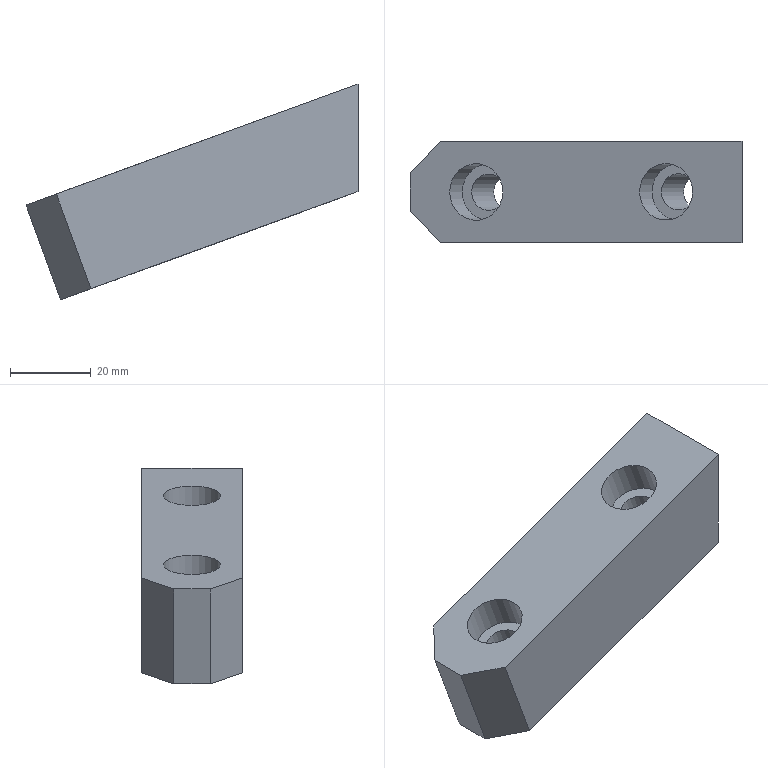Part | STEP file | P011002S003-009 | 1 solid | 14 faces | box 82.185 x 25 x 53.405 mm | volume 45412 mm3 | plane 10 | cylinder 4 | commonest cylinder face diameters 9 x2 14 x2
STEP:
#1=CARTESIAN_POINT('',(0.,0.,0.));
#2=DIRECTION('',(0.,0.,1.));
#3=DIRECTION('',(1.,0.,0.));
#4=AXIS2_PLACEMENT_3D('',#1,#2,#3);
#5=CARTESIAN_POINT('',(-226.457,-9.,-53.01));
#6=VERTEX_POINT('',#5);
#7=CARTESIAN_POINT('',(-217.999,-9.,-49.932));
#8=VERTEX_POINT('',#7);
#9=CARTESIAN_POINT('',(-222.228,-9.,-51.471));
#10=DIRECTION('',(0.342,0.,-0.9397));
#11=DIRECTION('',(-0.9397,0.,-0.342));
#12=AXIS2_PLACEMENT_3D('',#9,#10,#11);
#13=CIRCLE('',#12,4.5);
#14=CARTESIAN_POINT('',(-161.58,106.,-29.397));
#15=DIRECTION('',(0.342,0.,-0.9397));
#16=DIRECTION('',(0.9397,0.,0.342));
#17=AXIS2_PLACEMENT_3D('',#14,#15,#16);
#18=PLANE('',#17);
#19=CARTESIAN_POINT('',(-64.54,115.));
#20=DIRECTION('',(-1.,0.));
#21=AXIS2_PLACEMENT_2D('',#19,#20);
#22=CIRCLE('',#21,4.5);
#23=(GEOMETRIC_REPRESENTATION_CONTEXT(2)PARAMETRIC_REPRESENTATION_CONTEXT()REPRESENTATION_CONTEXT('',''));
#24=DEFINITIONAL_REPRESENTATION('',(#22),#23);
#25=PCURVE('',#18,#24);
#26=CARTESIAN_POINT('',(-230.778,-9.,-27.979));
#27=DIRECTION('',(0.342,0.,-0.9397));
#28=DIRECTION('',(0.9397,0.,0.342));
#29=AXIS2_PLACEMENT_3D('',#26,#27,#28);
#30=CYLINDRICAL_SURFACE('',#29,4.5);
#31=CARTESIAN_POINT('',(3.142,25.));
#32=DIRECTION('',(1.,0.));
#33=VECTOR('',#32,1.);
#34=LINE('',#31,#33);
#35=(GEOMETRIC_REPRESENTATION_CONTEXT(2)PARAMETRIC_REPRESENTATION_CONTEXT()REPRESENTATION_CONTEXT('',''));
#36=DEFINITIONAL_REPRESENTATION('',(#34),#35);
#37=PCURVE('',#30,#36);
#38=SURFACE_CURVE('',#13,(#25,#37),.PCURVE_S1.);
#39=EDGE_CURVE('',#6,#8,#38,.T.);
#40=ORIENTED_EDGE('',*,*,#39,.F.);
#41=CARTESIAN_POINT('',(-222.228,-9.,-51.471));
#42=DIRECTION('',(0.342,0.,-0.9397));
#43=DIRECTION('',(-0.9397,0.,-0.342));
#44=AXIS2_PLACEMENT_3D('',#41,#42,#43);
#45=CIRCLE('',#44,4.5);
#46=CARTESIAN_POINT('',(-64.54,115.));
#47=DIRECTION('',(-1.,0.));
#48=AXIS2_PLACEMENT_2D('',#46,#47);
#49=CIRCLE('',#48,4.5);
#50=(GEOMETRIC_REPRESENTATION_CONTEXT(2)PARAMETRIC_REPRESENTATION_CONTEXT()REPRESENTATION_CONTEXT('',''));
#51=DEFINITIONAL_REPRESENTATION('',(#49),#50);
#52=PCURVE('',#18,#51);
#53=CARTESIAN_POINT('',(-3.142,25.));
#54=DIRECTION('',(1.,0.));
#55=VECTOR('',#54,1.);
#56=LINE('',#53,#55);
#57=(GEOMETRIC_REPRESENTATION_CONTEXT(2)PARAMETRIC_REPRESENTATION_CONTEXT()REPRESENTATION_CONTEXT('',''));
#58=DEFINITIONAL_REPRESENTATION('',(#56),#57);
#59=PCURVE('',#30,#58);
#60=SURFACE_CURVE('',#45,(#52,#59),.PCURVE_S1.);
#61=EDGE_CURVE('',#8,#6,#60,.T.);
#62=ORIENTED_EDGE('',*,*,#61,.F.);
#63=EDGE_LOOP('',(#40,#62));
#64=FACE_BOUND('',#63,.T.);
#65=CARTESIAN_POINT('',(-165.,3.5,-30.642));
#66=VERTEX_POINT('',#65);
#67=CARTESIAN_POINT('',(-231.117,3.5,-54.706));
#68=VERTEX_POINT('',#67);
#69=CARTESIAN_POINT('',(-224.539,3.5,-52.312));
#70=DIRECTION('',(-0.9397,0.,-0.342));
#71=VECTOR('',#70,1.);
#72=LINE('',#69,#71);
#73=CARTESIAN_POINT('',(-67.,102.5));
#74=DIRECTION('',(-1.,0.));
#75=VECTOR('',#74,1.);
#76=LINE('',#73,#75);
#77=(GEOMETRIC_REPRESENTATION_CONTEXT(2)PARAMETRIC_REPRESENTATION_CONTEXT()REPRESENTATION_CONTEXT('',''));
#78=DEFINITIONAL_REPRESENTATION('',(#76),#77);
#79=PCURVE('',#18,#78);
#80=CARTESIAN_POINT('',(-229.67,3.5,-38.217));
#81=DIRECTION('',(0.,1.,0.));
#82=DIRECTION('',(0.9397,0.,0.342));
#83=AXIS2_PLACEMENT_3D('',#80,#81,#82);
#84=PLANE('',#83);
#85=CARTESIAN_POINT('',(0.,15.));
#86=DIRECTION('',(-1.,0.));
#87=VECTOR('',#86,1.);
#88=LINE('',#85,#87);
#89=(GEOMETRIC_REPRESENTATION_CONTEXT(2)PARAMETRIC_REPRESENTATION_CONTEXT()REPRESENTATION_CONTEXT('',''));
#90=DEFINITIONAL_REPRESENTATION('',(#88),#89);
#91=PCURVE('',#84,#90);
#92=SURFACE_CURVE('',#72,(#79,#91),.PCURVE_S1.);
#93=EDGE_CURVE('',#66,#68,#92,.T.);
#94=ORIENTED_EDGE('',*,*,#93,.F.);
#95=CARTESIAN_POINT('',(-165.,-21.5,-30.642));
#96=VERTEX_POINT('',#95);
#97=CARTESIAN_POINT('',(-165.,200.,-30.642));
#98=DIRECTION('',(0.,1.,0.));
#99=VECTOR('',#98,1.);
#100=LINE('',#97,#99);
#101=CARTESIAN_POINT('',(-3.64,-94.));
#102=DIRECTION('',(0.,-1.));
#103=VECTOR('',#102,1.);
#104=LINE('',#101,#103);
#105=(GEOMETRIC_REPRESENTATION_CONTEXT(2)PARAMETRIC_REPRESENTATION_CONTEXT()REPRESENTATION_CONTEXT('',''));
#106=DEFINITIONAL_REPRESENTATION('',(#104),#105);
#107=PCURVE('',#18,#106);
#108=CARTESIAN_POINT('',(-165.,200.,-50.));
#109=DIRECTION('',(1.,0.,0.));
#110=DIRECTION('',(0.,-1.,0.));
#111=AXIS2_PLACEMENT_3D('',#108,#109,#110);
#112=PLANE('',#111);
#113=CARTESIAN_POINT('',(0.,-19.358));
#114=DIRECTION('',(-1.,0.));
#115=VECTOR('',#114,1.);
#116=LINE('',#113,#115);
#117=(GEOMETRIC_REPRESENTATION_CONTEXT(2)PARAMETRIC_REPRESENTATION_CONTEXT()REPRESENTATION_CONTEXT('',''));
#118=DEFINITIONAL_REPRESENTATION('',(#116),#117);
#119=PCURVE('',#112,#118);
#120=SURFACE_CURVE('',#100,(#107,#119),.PCURVE_S1.);
#121=EDGE_CURVE('',#96,#66,#120,.T.);
#122=ORIENTED_EDGE('',*,*,#121,.F.);
#123=CARTESIAN_POINT('',(-231.117,-21.5,-54.706));
#124=VERTEX_POINT('',#123);
#125=CARTESIAN_POINT('',(-161.58,-21.5,-29.397));
#126=DIRECTION('',(-0.9397,0.,-0.342));
#127=VECTOR('',#126,1.);
#128=LINE('',#125,#127);
#129=CARTESIAN_POINT('',(0.,127.5));
#130=DIRECTION('',(-1.,0.));
#131=VECTOR('',#130,1.);
#132=LINE('',#129,#131);
#133=(GEOMETRIC_REPRESENTATION_CONTEXT(2)PARAMETRIC_REPRESENTATION_CONTEXT()REPRESENTATION_CONTEXT('',''));
#134=DEFINITIONAL_REPRESENTATION('',(#132),#133);
#135=PCURVE('',#18,#134);
#136=CARTESIAN_POINT('',(-229.67,-21.5,-38.217));
#137=DIRECTION('',(0.,-1.,0.));
#138=DIRECTION('',(-0.9397,0.,-0.342));
#139=AXIS2_PLACEMENT_3D('',#136,#137,#138);
#140=PLANE('',#139);
#141=CARTESIAN_POINT('',(-67.,15.));
#142=DIRECTION('',(1.,0.));
#143=VECTOR('',#142,1.);
#144=LINE('',#141,#143);
#145=(GEOMETRIC_REPRESENTATION_CONTEXT(2)PARAMETRIC_REPRESENTATION_CONTEXT()REPRESENTATION_CONTEXT('',''));
#146=DEFINITIONAL_REPRESENTATION('',(#144),#145);
#147=PCURVE('',#140,#146);
#148=SURFACE_CURVE('',#128,(#135,#147),.PCURVE_S1.);
#149=EDGE_CURVE('',#96,#124,#148,.T.);
#150=ORIENTED_EDGE('',*,*,#149,.T.);
#151=CARTESIAN_POINT('',(-238.635,-13.5,-57.443));
#152=VERTEX_POINT('',#151);
#153=CARTESIAN_POINT('',(-231.117,-21.5,-54.706));
#154=DIRECTION('',(0.6645,-0.7071,0.2418));
#155=VECTOR('',#154,1.);
#156=LINE('',#153,#155);
#157=CARTESIAN_POINT('',(-74.,127.5));
#158=DIRECTION('',(0.7071,0.7071));
#159=VECTOR('',#158,1.);
#160=LINE('',#157,#159);
#161=(GEOMETRIC_REPRESENTATION_CONTEXT(2)PARAMETRIC_REPRESENTATION_CONTEXT()REPRESENTATION_CONTEXT('',''));
#162=DEFINITIONAL_REPRESENTATION('',(#160),#161);
#163=PCURVE('',#18,#162);
#164=CARTESIAN_POINT('',(-236.247,-21.5,-40.611));
#165=DIRECTION('',(0.6645,0.7071,0.2418));
#166=DIRECTION('',(0.7287,-0.6848,0.));
#167=AXIS2_PLACEMENT_3D('',#164,#165,#166);
#168=PLANE('',#167);
#169=CARTESIAN_POINT('',(3.739,14.527));
#170=DIRECTION('',(0.9684,-0.2492));
#171=VECTOR('',#170,1.);
#172=LINE('',#169,#171);
#173=(GEOMETRIC_REPRESENTATION_CONTEXT(2)PARAMETRIC_REPRESENTATION_CONTEXT()REPRESENTATION_CONTEXT('',''));
#174=DEFINITIONAL_REPRESENTATION('',(#172),#173);
#175=PCURVE('',#168,#174);
#176=SURFACE_CURVE('',#156,(#163,#175),.PCURVE_S1.);
#177=EDGE_CURVE('',#152,#124,#176,.T.);
#178=ORIENTED_EDGE('',*,*,#177,.F.);
#179=CARTESIAN_POINT('',(-238.635,-4.5,-57.443));
#180=VERTEX_POINT('',#179);
#181=CARTESIAN_POINT('',(-238.635,-14.,-57.443));
#182=DIRECTION('',(0.,-1.,0.));
#183=VECTOR('',#182,1.);
#184=LINE('',#181,#183);
#185=CARTESIAN_POINT('',(-82.,120.));
#186=DIRECTION('',(0.,1.));
#187=VECTOR('',#186,1.);
#188=LINE('',#185,#187);
#189=(GEOMETRIC_REPRESENTATION_CONTEXT(2)PARAMETRIC_REPRESENTATION_CONTEXT()REPRESENTATION_CONTEXT('',''));
#190=DEFINITIONAL_REPRESENTATION('',(#188),#189);
#191=PCURVE('',#18,#190);
#192=CARTESIAN_POINT('',(-243.765,-14.,-43.347));
#193=DIRECTION('',(-0.9397,0.,-0.342));
#194=DIRECTION('',(-0.342,0.,0.9397));
#195=AXIS2_PLACEMENT_3D('',#192,#193,#194);
#196=PLANE('',#195);
#197=CARTESIAN_POINT('',(-15.,0.));
#198=DIRECTION('',(0.,-1.));
#199=VECTOR('',#198,1.);
#200=LINE('',#197,#199);
#201=(GEOMETRIC_REPRESENTATION_CONTEXT(2)PARAMETRIC_REPRESENTATION_CONTEXT()REPRESENTATION_CONTEXT('',''));
#202=DEFINITIONAL_REPRESENTATION('',(#200),#201);
#203=PCURVE('',#196,#202);
#204=SURFACE_CURVE('',#184,(#191,#203),.PCURVE_S1.);
#205=EDGE_CURVE('',#180,#152,#204,.T.);
#206=ORIENTED_EDGE('',*,*,#205,.F.);
#207=CARTESIAN_POINT('',(-231.117,3.5,-54.706));
#208=DIRECTION('',(-0.6645,-0.7071,-0.2418));
#209=VECTOR('',#208,1.);
#210=LINE('',#207,#209);
#211=CARTESIAN_POINT('',(-74.,102.5));
#212=DIRECTION('',(-0.7071,0.7071));
#213=VECTOR('',#212,1.);
#214=LINE('',#211,#213);
#215=(GEOMETRIC_REPRESENTATION_CONTEXT(2)PARAMETRIC_REPRESENTATION_CONTEXT()REPRESENTATION_CONTEXT('',''));
#216=DEFINITIONAL_REPRESENTATION('',(#214),#215);
#217=PCURVE('',#18,#216);
#218=CARTESIAN_POINT('',(-236.247,3.5,-40.611));
#219=DIRECTION('',(0.6645,-0.7071,0.2418));
#220=DIRECTION('',(-0.7287,-0.6848,0.));
#221=AXIS2_PLACEMENT_3D('',#218,#219,#220);
#222=PLANE('',#221);
#223=CARTESIAN_POINT('',(-3.739,14.527));
#224=DIRECTION('',(0.9684,0.2492));
#225=VECTOR('',#224,1.);
#226=LINE('',#223,#225);
#227=(GEOMETRIC_REPRESENTATION_CONTEXT(2)PARAMETRIC_REPRESENTATION_CONTEXT()REPRESENTATION_CONTEXT('',''));
#228=DEFINITIONAL_REPRESENTATION('',(#226),#227);
#229=PCURVE('',#222,#228);
#230=SURFACE_CURVE('',#210,(#217,#229),.PCURVE_S1.);
#231=EDGE_CURVE('',#68,#180,#230,.T.);
#232=ORIENTED_EDGE('',*,*,#231,.F.);
#233=EDGE_LOOP('',(#94,#122,#150,#178,#206,#232));
#234=FACE_BOUND('',#233,.T.);
#235=CARTESIAN_POINT('',(-179.472,-9.,-35.909));
#236=VERTEX_POINT('',#235);
#237=CARTESIAN_POINT('',(-171.015,-9.,-32.831));
#238=VERTEX_POINT('',#237);
#239=CARTESIAN_POINT('',(-175.243,-9.,-34.37));
#240=DIRECTION('',(0.342,0.,-0.9397));
#241=DIRECTION('',(-0.9397,0.,-0.342));
#242=AXIS2_PLACEMENT_3D('',#239,#240,#241);
#243=CIRCLE('',#242,4.5);
#244=CARTESIAN_POINT('',(-14.54,115.));
#245=DIRECTION('',(-1.,0.));
#246=AXIS2_PLACEMENT_2D('',#244,#245);
#247=CIRCLE('',#246,4.5);
#248=(GEOMETRIC_REPRESENTATION_CONTEXT(2)PARAMETRIC_REPRESENTATION_CONTEXT()REPRESENTATION_CONTEXT('',''));
#249=DEFINITIONAL_REPRESENTATION('',(#247),#248);
#250=PCURVE('',#18,#249);
#251=CARTESIAN_POINT('',(-183.794,-9.,-10.878));
#252=DIRECTION('',(0.342,0.,-0.9397));
#253=DIRECTION('',(0.9397,0.,0.342));
#254=AXIS2_PLACEMENT_3D('',#251,#252,#253);
#255=CYLINDRICAL_SURFACE('',#254,4.5);
#256=CARTESIAN_POINT('',(3.142,25.));
#257=DIRECTION('',(1.,0.));
#258=VECTOR('',#257,1.);
#259=LINE('',#256,#258);
#260=(GEOMETRIC_REPRESENTATION_CONTEXT(2)PARAMETRIC_REPRESENTATION_CONTEXT()REPRESENTATION_CONTEXT('',''));
#261=DEFINITIONAL_REPRESENTATION('',(#259),#260);
#262=PCURVE('',#255,#261);
#263=SURFACE_CURVE('',#243,(#250,#262),.PCURVE_S1.);
#264=EDGE_CURVE('',#236,#238,#263,.T.);
#265=ORIENTED_EDGE('',*,*,#264,.F.);
#266=CARTESIAN_POINT('',(-175.243,-9.,-34.37));
#267=DIRECTION('',(0.342,0.,-0.9397));
#268=DIRECTION('',(-0.9397,0.,-0.342));
#269=AXIS2_PLACEMENT_3D('',#266,#267,#268);
#270=CIRCLE('',#269,4.5);
#271=CARTESIAN_POINT('',(-14.54,115.));
#272=DIRECTION('',(-1.,0.));
#273=AXIS2_PLACEMENT_2D('',#271,#272);
#274=CIRCLE('',#273,4.5);
#275=(GEOMETRIC_REPRESENTATION_CONTEXT(2)PARAMETRIC_REPRESENTATION_CONTEXT()REPRESENTATION_CONTEXT('',''));
#276=DEFINITIONAL_REPRESENTATION('',(#274),#275);
#277=PCURVE('',#18,#276);
#278=CARTESIAN_POINT('',(-3.142,25.));
#279=DIRECTION('',(1.,0.));
#280=VECTOR('',#279,1.);
#281=LINE('',#278,#280);
#282=(GEOMETRIC_REPRESENTATION_CONTEXT(2)PARAMETRIC_REPRESENTATION_CONTEXT()REPRESENTATION_CONTEXT('',''));
#283=DEFINITIONAL_REPRESENTATION('',(#281),#282);
#284=PCURVE('',#255,#283);
#285=SURFACE_CURVE('',#270,(#277,#284),.PCURVE_S1.);
#286=EDGE_CURVE('',#238,#236,#285,.T.);
#287=ORIENTED_EDGE('',*,*,#286,.F.);
#288=EDGE_LOOP('',(#265,#287));
#289=FACE_BOUND('',#288,.T.);
#290=ADVANCED_FACE('',(#64,#234,#289),#18,.T.);
#291=ORIENTED_EDGE('',*,*,#205,.T.);
#292=CARTESIAN_POINT('',(-247.185,-13.5,-33.95));
#293=VERTEX_POINT('',#292);
#294=CARTESIAN_POINT('',(-243.765,-13.5,-43.347));
#295=DIRECTION('',(0.342,0.,-0.9397));
#296=VECTOR('',#295,1.);
#297=LINE('',#294,#296);
#298=CARTESIAN_POINT('',(0.,0.5));
#299=DIRECTION('',(-1.,0.));
#300=VECTOR('',#299,1.);
#301=LINE('',#298,#300);
#302=(GEOMETRIC_REPRESENTATION_CONTEXT(2)PARAMETRIC_REPRESENTATION_CONTEXT()REPRESENTATION_CONTEXT('',''));
#303=DEFINITIONAL_REPRESENTATION('',(#301),#302);
#304=PCURVE('',#196,#303);
#305=CARTESIAN_POINT('',(-10.957,2.82));
#306=DIRECTION('',(0.2492,0.9684));
#307=VECTOR('',#306,1.);
#308=LINE('',#305,#307);
#309=(GEOMETRIC_REPRESENTATION_CONTEXT(2)PARAMETRIC_REPRESENTATION_CONTEXT()REPRESENTATION_CONTEXT('',''));
#310=DEFINITIONAL_REPRESENTATION('',(#308),#309);
#311=PCURVE('',#168,#310);
#312=SURFACE_CURVE('',#297,(#304,#311),.PCURVE_S1.);
#313=EDGE_CURVE('',#293,#152,#312,.T.);
#314=ORIENTED_EDGE('',*,*,#313,.F.);
#315=CARTESIAN_POINT('',(-247.185,-4.5,-33.95));
#316=VERTEX_POINT('',#315);
#317=CARTESIAN_POINT('',(-247.185,-14.,-33.95));
#318=DIRECTION('',(0.,1.,0.));
#319=VECTOR('',#318,1.);
#320=LINE('',#317,#319);
#321=CARTESIAN_POINT('',(10.,0.));
#322=DIRECTION('',(0.,1.));
#323=VECTOR('',#322,1.);
#324=LINE('',#321,#323);
#325=(GEOMETRIC_REPRESENTATION_CONTEXT(2)PARAMETRIC_REPRESENTATION_CONTEXT()REPRESENTATION_CONTEXT('',''));
#326=DEFINITIONAL_REPRESENTATION('',(#324),#325);
#327=PCURVE('',#196,#326);
#328=CARTESIAN_POINT('',(-233.09,-14.,-28.82));
#329=DIRECTION('',(-0.342,0.,0.9397));
#330=DIRECTION('',(0.9397,0.,0.342));
#331=AXIS2_PLACEMENT_3D('',#328,#329,#330);
#332=PLANE('',#331);
#333=CARTESIAN_POINT('',(-15.,0.));
#334=DIRECTION('',(0.,1.));
#335=VECTOR('',#334,1.);
#336=LINE('',#333,#335);
#337=(GEOMETRIC_REPRESENTATION_CONTEXT(2)PARAMETRIC_REPRESENTATION_CONTEXT()REPRESENTATION_CONTEXT('',''));
#338=DEFINITIONAL_REPRESENTATION('',(#336),#337);
#339=PCURVE('',#332,#338);
#340=SURFACE_CURVE('',#320,(#327,#339),.PCURVE_S1.);
#341=EDGE_CURVE('',#293,#316,#340,.T.);
#342=ORIENTED_EDGE('',*,*,#341,.T.);
#343=CARTESIAN_POINT('',(-243.765,-4.5,-43.347));
#344=DIRECTION('',(-0.342,0.,0.9397));
#345=VECTOR('',#344,1.);
#346=LINE('',#343,#345);
#347=CARTESIAN_POINT('',(0.,9.5));
#348=DIRECTION('',(1.,0.));
#349=VECTOR('',#348,1.);
#350=LINE('',#347,#349);
#351=(GEOMETRIC_REPRESENTATION_CONTEXT(2)PARAMETRIC_REPRESENTATION_CONTEXT()REPRESENTATION_CONTEXT('',''));
#352=DEFINITIONAL_REPRESENTATION('',(#350),#351);
#353=PCURVE('',#196,#352);
#354=CARTESIAN_POINT('',(10.957,2.82));
#355=DIRECTION('',(0.2492,-0.9684));
#356=VECTOR('',#355,1.);
#357=LINE('',#354,#356);
#358=(GEOMETRIC_REPRESENTATION_CONTEXT(2)PARAMETRIC_REPRESENTATION_CONTEXT()REPRESENTATION_CONTEXT('',''));
#359=DEFINITIONAL_REPRESENTATION('',(#357),#358);
#360=PCURVE('',#222,#359);
#361=SURFACE_CURVE('',#346,(#353,#360),.PCURVE_S1.);
#362=EDGE_CURVE('',#180,#316,#361,.T.);
#363=ORIENTED_EDGE('',*,*,#362,.F.);
#364=EDGE_LOOP('',(#291,#314,#342,#363));
#365=FACE_BOUND('',#364,.T.);
#366=ADVANCED_FACE('',(#365),#196,.T.);
#367=CARTESIAN_POINT('',(-165.,3.5,-4.037));
#368=VERTEX_POINT('',#367);
#369=CARTESIAN_POINT('',(-239.668,3.5,-31.214));
#370=VERTEX_POINT('',#369);
#371=CARTESIAN_POINT('',(-233.09,3.5,-28.82));
#372=DIRECTION('',(-0.9397,0.,-0.342));
#373=VECTOR('',#372,1.);
#374=LINE('',#371,#373);
#375=CARTESIAN_POINT('',(0.,-10.));
#376=DIRECTION('',(-1.,0.));
#377=VECTOR('',#376,1.);
#378=LINE('',#375,#377);
#379=(GEOMETRIC_REPRESENTATION_CONTEXT(2)PARAMETRIC_REPRESENTATION_CONTEXT()REPRESENTATION_CONTEXT('',''));
#380=DEFINITIONAL_REPRESENTATION('',(#378),#379);
#381=PCURVE('',#84,#380);
#382=CARTESIAN_POINT('',(0.,17.5));
#383=DIRECTION('',(-1.,0.));
#384=VECTOR('',#383,1.);
#385=LINE('',#382,#384);
#386=(GEOMETRIC_REPRESENTATION_CONTEXT(2)PARAMETRIC_REPRESENTATION_CONTEXT()REPRESENTATION_CONTEXT('',''));
#387=DEFINITIONAL_REPRESENTATION('',(#385),#386);
#388=PCURVE('',#332,#387);
#389=SURFACE_CURVE('',#374,(#381,#388),.PCURVE_S1.);
#390=EDGE_CURVE('',#368,#370,#389,.T.);
#391=ORIENTED_EDGE('',*,*,#390,.F.);
#392=CARTESIAN_POINT('',(-165.,3.5,-38.217));
#393=DIRECTION('',(0.,0.,1.));
#394=VECTOR('',#393,1.);
#395=LINE('',#392,#394);
#396=CARTESIAN_POINT('',(60.769,22.118));
#397=DIRECTION('',(0.342,-0.9397));
#398=VECTOR('',#397,1.);
#399=LINE('',#396,#398);
#400=(GEOMETRIC_REPRESENTATION_CONTEXT(2)PARAMETRIC_REPRESENTATION_CONTEXT()REPRESENTATION_CONTEXT('',''));
#401=DEFINITIONAL_REPRESENTATION('',(#399),#400);
#402=PCURVE('',#84,#401);
#403=CARTESIAN_POINT('',(196.5,-11.783));
#404=DIRECTION('',(0.,-1.));
#405=VECTOR('',#404,1.);
#406=LINE('',#403,#405);
#407=(GEOMETRIC_REPRESENTATION_CONTEXT(2)PARAMETRIC_REPRESENTATION_CONTEXT()REPRESENTATION_CONTEXT('',''));
#408=DEFINITIONAL_REPRESENTATION('',(#406),#407);
#409=PCURVE('',#112,#408);
#410=SURFACE_CURVE('',#395,(#402,#409),.PCURVE_S1.);
#411=EDGE_CURVE('',#66,#368,#410,.T.);
#412=ORIENTED_EDGE('',*,*,#411,.F.);
#413=ORIENTED_EDGE('',*,*,#93,.T.);
#414=CARTESIAN_POINT('',(-236.247,3.5,-40.611));
#415=DIRECTION('',(0.342,0.,-0.9397));
#416=VECTOR('',#415,1.);
#417=LINE('',#414,#416);
#418=CARTESIAN_POINT('',(-7.,0.));
#419=DIRECTION('',(0.,1.));
#420=VECTOR('',#419,1.);
#421=LINE('',#418,#420);
#422=(GEOMETRIC_REPRESENTATION_CONTEXT(2)PARAMETRIC_REPRESENTATION_CONTEXT()REPRESENTATION_CONTEXT('',''));
#423=DEFINITIONAL_REPRESENTATION('',(#421),#422);
#424=PCURVE('',#84,#423);
#425=CARTESIAN_POINT('',(0.,0.));
#426=DIRECTION('',(-0.2492,0.9684));
#427=VECTOR('',#426,1.);
#428=LINE('',#425,#427);
#429=(GEOMETRIC_REPRESENTATION_CONTEXT(2)PARAMETRIC_REPRESENTATION_CONTEXT()REPRESENTATION_CONTEXT('',''));
#430=DEFINITIONAL_REPRESENTATION('',(#428),#429);
#431=PCURVE('',#222,#430);
#432=SURFACE_CURVE('',#417,(#424,#431),.PCURVE_S1.);
#433=EDGE_CURVE('',#370,#68,#432,.T.);
#434=ORIENTED_EDGE('',*,*,#433,.F.);
#435=EDGE_LOOP('',(#391,#412,#413,#434));
#436=FACE_BOUND('',#435,.T.);
#437=ADVANCED_FACE('',(#436),#84,.T.);
#438=ORIENTED_EDGE('',*,*,#149,.F.);
#439=CARTESIAN_POINT('',(-165.,-21.5,-4.037));
#440=VERTEX_POINT('',#439);
#441=CARTESIAN_POINT('',(-165.,-21.5,-38.217));
#442=DIRECTION('',(0.,0.,-1.));
#443=VECTOR('',#442,1.);
#444=LINE('',#441,#443);
#445=CARTESIAN_POINT('',(-60.769,22.118));
#446=DIRECTION('',(0.342,0.9397));
#447=VECTOR('',#446,1.);
#448=LINE('',#445,#447);
#449=(GEOMETRIC_REPRESENTATION_CONTEXT(2)PARAMETRIC_REPRESENTATION_CONTEXT()REPRESENTATION_CONTEXT('',''));
#450=DEFINITIONAL_REPRESENTATION('',(#448),#449);
#451=PCURVE('',#140,#450);
#452=CARTESIAN_POINT('',(221.5,-11.783));
#453=DIRECTION('',(0.,1.));
#454=VECTOR('',#453,1.);
#455=LINE('',#452,#454);
#456=(GEOMETRIC_REPRESENTATION_CONTEXT(2)PARAMETRIC_REPRESENTATION_CONTEXT()REPRESENTATION_CONTEXT('',''));
#457=DEFINITIONAL_REPRESENTATION('',(#455),#456);
#458=PCURVE('',#112,#457);
#459=SURFACE_CURVE('',#444,(#451,#458),.PCURVE_S1.);
#460=EDGE_CURVE('',#440,#96,#459,.T.);
#461=ORIENTED_EDGE('',*,*,#460,.F.);
#462=CARTESIAN_POINT('',(-239.668,-21.5,-31.214));
#463=VERTEX_POINT('',#462);
#464=CARTESIAN_POINT('',(-233.09,-21.5,-28.82));
#465=DIRECTION('',(-0.9397,0.,-0.342));
#466=VECTOR('',#465,1.);
#467=LINE('',#464,#466);
#468=CARTESIAN_POINT('',(0.,-10.));
#469=DIRECTION('',(1.,0.));
#470=VECTOR('',#469,1.);
#471=LINE('',#468,#470);
#472=(GEOMETRIC_REPRESENTATION_CONTEXT(2)PARAMETRIC_REPRESENTATION_CONTEXT()REPRESENTATION_CONTEXT('',''));
#473=DEFINITIONAL_REPRESENTATION('',(#471),#472);
#474=PCURVE('',#140,#473);
#475=CARTESIAN_POINT('',(0.,-7.5));
#476=DIRECTION('',(-1.,0.));
#477=VECTOR('',#476,1.);
#478=LINE('',#475,#477);
#479=(GEOMETRIC_REPRESENTATION_CONTEXT(2)PARAMETRIC_REPRESENTATION_CONTEXT()REPRESENTATION_CONTEXT('',''));
#480=DEFINITIONAL_REPRESENTATION('',(#478),#479);
#481=PCURVE('',#332,#480);
#482=SURFACE_CURVE('',#467,(#474,#481),.PCURVE_S1.);
#483=EDGE_CURVE('',#440,#463,#482,.T.);
#484=ORIENTED_EDGE('',*,*,#483,.T.);
#485=CARTESIAN_POINT('',(-236.247,-21.5,-40.611));
#486=DIRECTION('',(-0.342,0.,0.9397));
#487=VECTOR('',#486,1.);
#488=LINE('',#485,#487);
#489=CARTESIAN_POINT('',(7.,0.));
#490=DIRECTION('',(0.,-1.));
#491=VECTOR('',#490,1.);
#492=LINE('',#489,#491);
#493=(GEOMETRIC_REPRESENTATION_CONTEXT(2)PARAMETRIC_REPRESENTATION_CONTEXT()REPRESENTATION_CONTEXT('',''));
#494=DEFINITIONAL_REPRESENTATION('',(#492),#493);
#495=PCURVE('',#140,#494);
#496=CARTESIAN_POINT('',(0.,0.));
#497=DIRECTION('',(-0.2492,-0.9684));
#498=VECTOR('',#497,1.);
#499=LINE('',#496,#498);
#500=(GEOMETRIC_REPRESENTATION_CONTEXT(2)PARAMETRIC_REPRESENTATION_CONTEXT()REPRESENTATION_CONTEXT('',''));
#501=DEFINITIONAL_REPRESENTATION('',(#499),#500);
#502=PCURVE('',#168,#501);
#503=SURFACE_CURVE('',#488,(#495,#502),.PCURVE_S1.);
#504=EDGE_CURVE('',#124,#463,#503,.T.);
#505=ORIENTED_EDGE('',*,*,#504,.F.);
#506=EDGE_LOOP('',(#438,#461,#484,#505));
#507=FACE_BOUND('',#506,.T.);
#508=ADVANCED_FACE('',(#507),#140,.T.);
#509=CARTESIAN_POINT('',(-165.,-14.,-4.037));
#510=DIRECTION('',(0.,-1.,0.));
#511=VECTOR('',#510,1.);
#512=LINE('',#509,#511);
#513=CARTESIAN_POINT('',(214.,-45.963));
#514=DIRECTION('',(1.,0.));
#515=VECTOR('',#514,1.);
#516=LINE('',#513,#515);
#517=(GEOMETRIC_REPRESENTATION_CONTEXT(2)PARAMETRIC_REPRESENTATION_CONTEXT()REPRESENTATION_CONTEXT('',''));
#518=DEFINITIONAL_REPRESENTATION('',(#516),#517);
#519=PCURVE('',#112,#518);
#520=CARTESIAN_POINT('',(72.46,0.));
#521=DIRECTION('',(0.,-1.));
#522=VECTOR('',#521,1.);
#523=LINE('',#520,#522);
#524=(GEOMETRIC_REPRESENTATION_CONTEXT(2)PARAMETRIC_REPRESENTATION_CONTEXT()REPRESENTATION_CONTEXT('',''));
#525=DEFINITIONAL_REPRESENTATION('',(#523),#524);
#526=PCURVE('',#332,#525);
#527=SURFACE_CURVE('',#512,(#519,#526),.PCURVE_S1.);
#528=EDGE_CURVE('',#368,#440,#527,.T.);
#529=ORIENTED_EDGE('',*,*,#528,.T.);
#530=ORIENTED_EDGE('',*,*,#460,.T.);
#531=ORIENTED_EDGE('',*,*,#121,.T.);
#532=ORIENTED_EDGE('',*,*,#411,.T.);
#533=EDGE_LOOP('',(#529,#530,#531,#532));
#534=FACE_BOUND('',#533,.T.);
#535=ADVANCED_FACE('',(#534),#112,.T.);
#536=CARTESIAN_POINT('',(-224.201,-9.,-25.585));
#537=VERTEX_POINT('',#536);
#538=CARTESIAN_POINT('',(-230.778,-9.,-27.979));
#539=DIRECTION('',(0.342,0.,-0.9397));
#540=DIRECTION('',(0.9397,0.,0.342));
#541=AXIS2_PLACEMENT_3D('',#538,#539,#540);
#542=CIRCLE('',#541,7.);
#543=CARTESIAN_POINT('',(9.46,5.));
#544=CARTESIAN_POINT('',(9.46,-7.124));
#545=CARTESIAN_POINT('',(-1.04,-1.062));
#546=CARTESIAN_POINT('',(-11.54,5.));
#547=CARTESIAN_POINT('',(-1.04,11.062));
#548=CARTESIAN_POINT('',(9.46,17.124));
#549=CARTESIAN_POINT('',(9.46,5.));
#550=(BOUNDED_CURVE()B_SPLINE_CURVE(2,(#543,#544,#545,#546,#547,#548,#549),.UNSPECIFIED.,.T.,.F.)B_SPLINE_CURVE_WITH_KNOTS((1,2,2,2,2,1),(-2.094,0.,2.094,4.189,6.283,8.378),.UNSPECIFIED.)CURVE()GEOMETRIC_REPRESENTATION_ITEM()RATIONAL_B_SPLINE_CURVE((1.,0.5,1.,0.5,1.,0.5,1.))REPRESENTATION_ITEM(''));
#551=(GEOMETRIC_REPRESENTATION_CONTEXT(2)PARAMETRIC_REPRESENTATION_CONTEXT()REPRESENTATION_CONTEXT('',''));
#552=DEFINITIONAL_REPRESENTATION('',(#550),#551);
#553=PCURVE('',#332,#552);
#554=CARTESIAN_POINT('',(-230.778,-9.,-27.979));
#555=DIRECTION('',(0.342,0.,-0.9397));
#556=DIRECTION('',(0.9397,0.,0.342));
#557=AXIS2_PLACEMENT_3D('',#554,#555,#556);
#558=CYLINDRICAL_SURFACE('',#557,7.);
#559=CARTESIAN_POINT('',(0.,0.));
#560=DIRECTION('',(1.,0.));
#561=VECTOR('',#560,1.);
#562=LINE('',#559,#561);
#563=(GEOMETRIC_REPRESENTATION_CONTEXT(2)PARAMETRIC_REPRESENTATION_CONTEXT()REPRESENTATION_CONTEXT('',''));
#564=DEFINITIONAL_REPRESENTATION('',(#562),#563);
#565=PCURVE('',#558,#564);
#566=SURFACE_CURVE('',#542,(#553,#565),.PCURVE_S1.);
#567=EDGE_CURVE('',#537,#537,#566,.T.);
#568=ORIENTED_EDGE('',*,*,#567,.T.);
#569=EDGE_LOOP('',(#568));
#570=FACE_BOUND('',#569,.T.);
#571=CARTESIAN_POINT('',(-177.216,-9.,-8.484));
#572=VERTEX_POINT('',#571);
#573=CARTESIAN_POINT('',(-183.794,-9.,-10.878));
#574=DIRECTION('',(0.342,0.,-0.9397));
#575=DIRECTION('',(0.9397,0.,0.342));
#576=AXIS2_PLACEMENT_3D('',#573,#574,#575);
#577=CIRCLE('',#576,7.);
#578=CARTESIAN_POINT('',(59.46,5.));
#579=CARTESIAN_POINT('',(59.46,-7.124));
#580=CARTESIAN_POINT('',(48.96,-1.062));
#581=CARTESIAN_POINT('',(38.46,5.));
#582=CARTESIAN_POINT('',(48.96,11.062));
#583=CARTESIAN_POINT('',(59.46,17.124));
#584=CARTESIAN_POINT('',(59.46,5.));
#585=(BOUNDED_CURVE()B_SPLINE_CURVE(2,(#578,#579,#580,#581,#582,#583,#584),.UNSPECIFIED.,.T.,.F.)B_SPLINE_CURVE_WITH_KNOTS((1,2,2,2,2,1),(-2.094,0.,2.094,4.189,6.283,8.378),.UNSPECIFIED.)CURVE()GEOMETRIC_REPRESENTATION_ITEM()RATIONAL_B_SPLINE_CURVE((1.,0.5,1.,0.5,1.,0.5,1.))REPRESENTATION_ITEM(''));
#586=(GEOMETRIC_REPRESENTATION_CONTEXT(2)PARAMETRIC_REPRESENTATION_CONTEXT()REPRESENTATION_CONTEXT('',''));
#587=DEFINITIONAL_REPRESENTATION('',(#585),#586);
#588=PCURVE('',#332,#587);
#589=CARTESIAN_POINT('',(-183.794,-9.,-10.878));
#590=DIRECTION('',(0.342,0.,-0.9397));
#591=DIRECTION('',(0.9397,0.,0.342));
#592=AXIS2_PLACEMENT_3D('',#589,#590,#591);
#593=CYLINDRICAL_SURFACE('',#592,7.);
#594=CARTESIAN_POINT('',(0.,0.));
#595=DIRECTION('',(1.,0.));
#596=VECTOR('',#595,1.);
#597=LINE('',#594,#596);
#598=(GEOMETRIC_REPRESENTATION_CONTEXT(2)PARAMETRIC_REPRESENTATION_CONTEXT()REPRESENTATION_CONTEXT('',''));
#599=DEFINITIONAL_REPRESENTATION('',(#597),#598);
#600=PCURVE('',#593,#599);
#601=SURFACE_CURVE('',#577,(#588,#600),.PCURVE_S1.);
#602=EDGE_CURVE('',#572,#572,#601,.T.);
#603=ORIENTED_EDGE('',*,*,#602,.T.);
#604=EDGE_LOOP('',(#603));
#605=FACE_BOUND('',#604,.T.);
#606=ORIENTED_EDGE('',*,*,#341,.F.);
#607=CARTESIAN_POINT('',(-239.902,-21.25,-31.3));
#608=DIRECTION('',(-0.6645,0.7071,-0.2418));
#609=VECTOR('',#608,1.);
#610=LINE('',#607,#609);
#611=CARTESIAN_POINT('',(-7.25,-7.25));
#612=DIRECTION('',(-0.7071,0.7071));
#613=VECTOR('',#612,1.);
#614=LINE('',#611,#613);
#615=(GEOMETRIC_REPRESENTATION_CONTEXT(2)PARAMETRIC_REPRESENTATION_CONTEXT()REPRESENTATION_CONTEXT('',''));
#616=DEFINITIONAL_REPRESENTATION('',(#614),#615);
#617=PCURVE('',#332,#616);
#618=CARTESIAN_POINT('',(-2.835,-9.596));
#619=DIRECTION('',(-0.9684,0.2492));
#620=VECTOR('',#619,1.);
#621=LINE('',#618,#620);
#622=(GEOMETRIC_REPRESENTATION_CONTEXT(2)PARAMETRIC_REPRESENTATION_CONTEXT()REPRESENTATION_CONTEXT('',''));
#623=DEFINITIONAL_REPRESENTATION('',(#621),#622);
#624=PCURVE('',#168,#623);
#625=SURFACE_CURVE('',#610,(#617,#624),.PCURVE_S1.);
#626=EDGE_CURVE('',#463,#293,#625,.T.);
#627=ORIENTED_EDGE('',*,*,#626,.F.);
#628=ORIENTED_EDGE('',*,*,#483,.F.);
#629=ORIENTED_EDGE('',*,*,#528,.F.);
#630=ORIENTED_EDGE('',*,*,#390,.T.);
#631=CARTESIAN_POINT('',(-244.601,-1.75,-33.01));
#632=DIRECTION('',(0.6645,0.7071,0.2418));
#633=VECTOR('',#632,1.);
#634=LINE('',#631,#633);
#635=CARTESIAN_POINT('',(-12.25,12.25));
#636=DIRECTION('',(0.7071,0.7071));
#637=VECTOR('',#636,1.);
#638=LINE('',#635,#637);
#639=(GEOMETRIC_REPRESENTATION_CONTEXT(2)PARAMETRIC_REPRESENTATION_CONTEXT()REPRESENTATION_CONTEXT('',''));
#640=DEFINITIONAL_REPRESENTATION('',(#638),#639);
#641=PCURVE('',#332,#640);
#642=CARTESIAN_POINT('',(9.683,-7.834));
#643=DIRECTION('',(-0.9684,-0.2492));
#644=VECTOR('',#643,1.);
#645=LINE('',#642,#644);
#646=(GEOMETRIC_REPRESENTATION_CONTEXT(2)PARAMETRIC_REPRESENTATION_CONTEXT()REPRESENTATION_CONTEXT('',''));
#647=DEFINITIONAL_REPRESENTATION('',(#645),#646);
#648=PCURVE('',#222,#647);
#649=SURFACE_CURVE('',#634,(#641,#648),.PCURVE_S1.);
#650=EDGE_CURVE('',#316,#370,#649,.T.);
#651=ORIENTED_EDGE('',*,*,#650,.F.);
#652=EDGE_LOOP('',(#606,#627,#628,#629,#630,#651));
#653=FACE_BOUND('',#652,.T.);
#654=ADVANCED_FACE('',(#570,#605,#653),#332,.T.);
#655=ORIENTED_EDGE('',*,*,#650,.T.);
#656=ORIENTED_EDGE('',*,*,#433,.T.);
#657=ORIENTED_EDGE('',*,*,#231,.T.);
#658=ORIENTED_EDGE('',*,*,#362,.T.);
#659=EDGE_LOOP('',(#655,#656,#657,#658));
#660=FACE_BOUND('',#659,.T.);
#661=ADVANCED_FACE('',(#660),#222,.F.);
#662=ORIENTED_EDGE('',*,*,#177,.T.);
#663=ORIENTED_EDGE('',*,*,#504,.T.);
#664=ORIENTED_EDGE('',*,*,#626,.T.);
#665=ORIENTED_EDGE('',*,*,#313,.T.);
#666=EDGE_LOOP('',(#662,#663,#664,#665));
#667=FACE_BOUND('',#666,.T.);
#668=ADVANCED_FACE('',(#667),#168,.F.);
#669=ORIENTED_EDGE('',*,*,#286,.F.);
#670=CARTESIAN_POINT('',(-176.487,-9.,-17.796));
#671=VERTEX_POINT('',#670);
#672=CARTESIAN_POINT('',(-176.487,-9.,-17.796));
#673=CARTESIAN_POINT('',(-171.015,-9.,-32.831));
#674=B_SPLINE_CURVE_WITH_KNOTS('',1,(#672,#673),.UNSPECIFIED.,.F.,.F.,(2,2),(9.,25.),.PIECEWISE_BEZIER_KNOTS.);
#675=CARTESIAN_POINT('',(0.,0.));
#676=DIRECTION('',(0.,1.));
#677=VECTOR('',#676,1.);
#678=LINE('',#675,#677);
#679=(GEOMETRIC_REPRESENTATION_CONTEXT(2)PARAMETRIC_REPRESENTATION_CONTEXT()REPRESENTATION_CONTEXT('',''));
#680=DEFINITIONAL_REPRESENTATION('',(#678),#679);
#681=PCURVE('',#255,#680);
#682=CARTESIAN_POINT('',(6.283,0.));
#683=DIRECTION('',(0.,1.));
#684=VECTOR('',#683,1.);
#685=LINE('',#682,#684);
#686=(GEOMETRIC_REPRESENTATION_CONTEXT(2)PARAMETRIC_REPRESENTATION_CONTEXT()REPRESENTATION_CONTEXT('',''));
#687=DEFINITIONAL_REPRESENTATION('',(#685),#686);
#688=PCURVE('',#255,#687);
#689=SEAM_CURVE('',#674,(#681,#688),.PCURVE_S1.);
#690=EDGE_CURVE('',#671,#238,#689,.T.);
#691=ORIENTED_EDGE('',*,*,#690,.F.);
#692=CARTESIAN_POINT('',(-180.716,-9.,-19.335));
#693=DIRECTION('',(-0.342,0.,0.9397));
#694=DIRECTION('',(0.9397,0.,0.342));
#695=AXIS2_PLACEMENT_3D('',#692,#693,#694);
#696=CIRCLE('',#695,4.5);
#697=CARTESIAN_POINT('',(6.283,9.));
#698=DIRECTION('',(-1.,0.));
#699=VECTOR('',#698,1.);
#700=LINE('',#697,#699);
#701=(GEOMETRIC_REPRESENTATION_CONTEXT(2)PARAMETRIC_REPRESENTATION_CONTEXT()REPRESENTATION_CONTEXT('',''));
#702=DEFINITIONAL_REPRESENTATION('',(#700),#701);
#703=PCURVE('',#255,#702);
#704=CARTESIAN_POINT('',(-176.017,-9.,-17.625));
#705=DIRECTION('',(0.342,0.,-0.9397));
#706=DIRECTION('',(0.9397,0.,0.342));
#707=AXIS2_PLACEMENT_3D('',#704,#705,#706);
#708=PLANE('',#707);
#709=CARTESIAN_POINT('',(-0.5,0.));
#710=CARTESIAN_POINT('',(-0.5,-7.794));
#711=CARTESIAN_POINT('',(-7.25,-3.897));
#712=CARTESIAN_POINT('',(-14.,0.));
#713=CARTESIAN_POINT('',(-7.25,3.897));
#714=CARTESIAN_POINT('',(-0.5,7.794));
#715=CARTESIAN_POINT('',(-0.5,0.));
#716=(BOUNDED_CURVE()B_SPLINE_CURVE(2,(#709,#710,#711,#712,#713,#714,#715),.UNSPECIFIED.,.T.,.F.)B_SPLINE_CURVE_WITH_KNOTS((1,2,2,2,2,1),(-2.094,0.,2.094,4.189,6.283,8.378),.UNSPECIFIED.)CURVE()GEOMETRIC_REPRESENTATION_ITEM()RATIONAL_B_SPLINE_CURVE((1.,0.5,1.,0.5,1.,0.5,1.))REPRESENTATION_ITEM(''));
#717=(GEOMETRIC_REPRESENTATION_CONTEXT(2)PARAMETRIC_REPRESENTATION_CONTEXT()REPRESENTATION_CONTEXT('',''));
#718=DEFINITIONAL_REPRESENTATION('',(#716),#717);
#719=PCURVE('',#708,#718);
#720=SURFACE_CURVE('',#696,(#703,#719),.PCURVE_S1.);
#721=EDGE_CURVE('',#671,#671,#720,.T.);
#722=ORIENTED_EDGE('',*,*,#721,.F.);
#723=ORIENTED_EDGE('',*,*,#690,.T.);
#724=ORIENTED_EDGE('',*,*,#264,.F.);
#725=EDGE_LOOP('',(#669,#691,#722,#723,#724));
#726=FACE_BOUND('',#725,.F.);
#727=ADVANCED_FACE('',(#726),#255,.F.);
#728=CARTESIAN_POINT('',(-174.138,-9.,-16.941));
#729=VERTEX_POINT('',#728);
#730=CARTESIAN_POINT('',(-180.716,-9.,-19.335));
#731=DIRECTION('',(-0.342,0.,0.9397));
#732=DIRECTION('',(0.9397,0.,0.342));
#733=AXIS2_PLACEMENT_3D('',#730,#731,#732);
#734=CIRCLE('',#733,7.);
#735=CARTESIAN_POINT('',(2.,0.));
#736=CARTESIAN_POINT('',(2.,-12.124));
#737=CARTESIAN_POINT('',(-8.5,-6.062));
#738=CARTESIAN_POINT('',(-19.,0.));
#739=CARTESIAN_POINT('',(-8.5,6.062));
#740=CARTESIAN_POINT('',(2.,12.124));
#741=CARTESIAN_POINT('',(2.,0.));
#742=(BOUNDED_CURVE()B_SPLINE_CURVE(2,(#735,#736,#737,#738,#739,#740,#741),.UNSPECIFIED.,.T.,.F.)B_SPLINE_CURVE_WITH_KNOTS((1,2,2,2,2,1),(-2.094,0.,2.094,4.189,6.283,8.378),.UNSPECIFIED.)CURVE()GEOMETRIC_REPRESENTATION_ITEM()RATIONAL_B_SPLINE_CURVE((1.,0.5,1.,0.5,1.,0.5,1.))REPRESENTATION_ITEM(''));
#743=(GEOMETRIC_REPRESENTATION_CONTEXT(2)PARAMETRIC_REPRESENTATION_CONTEXT()REPRESENTATION_CONTEXT('',''));
#744=DEFINITIONAL_REPRESENTATION('',(#742),#743);
#745=PCURVE('',#708,#744);
#746=CARTESIAN_POINT('',(6.283,9.));
#747=DIRECTION('',(-1.,0.));
#748=VECTOR('',#747,1.);
#749=LINE('',#746,#748);
#750=(GEOMETRIC_REPRESENTATION_CONTEXT(2)PARAMETRIC_REPRESENTATION_CONTEXT()REPRESENTATION_CONTEXT('',''));
#751=DEFINITIONAL_REPRESENTATION('',(#749),#750);
#752=PCURVE('',#593,#751);
#753=SURFACE_CURVE('',#734,(#745,#752),.PCURVE_S1.);
#754=EDGE_CURVE('',#729,#729,#753,.T.);
#755=ORIENTED_EDGE('',*,*,#754,.T.);
#756=EDGE_LOOP('',(#755));
#757=FACE_BOUND('',#756,.T.);
#758=ORIENTED_EDGE('',*,*,#721,.F.);
#759=EDGE_LOOP('',(#758));
#760=FACE_BOUND('',#759,.T.);
#761=ADVANCED_FACE('',(#757,#760),#708,.F.);
#762=ORIENTED_EDGE('',*,*,#602,.T.);
#763=CARTESIAN_POINT('',(-177.216,-9.,-8.484));
#764=CARTESIAN_POINT('',(-174.138,-9.,-16.941));
#765=B_SPLINE_CURVE_WITH_KNOTS('',1,(#763,#764),.UNSPECIFIED.,.F.,.F.,(2,2),(0.,9.),.PIECEWISE_BEZIER_KNOTS.);
#766=CARTESIAN_POINT('',(6.283,0.));
#767=DIRECTION('',(0.,1.));
#768=VECTOR('',#767,1.);
#769=LINE('',#766,#768);
#770=(GEOMETRIC_REPRESENTATION_CONTEXT(2)PARAMETRIC_REPRESENTATION_CONTEXT()REPRESENTATION_CONTEXT('',''));
#771=DEFINITIONAL_REPRESENTATION('',(#769),#770);
#772=PCURVE('',#593,#771);
#773=CARTESIAN_POINT('',(0.,0.));
#774=DIRECTION('',(0.,1.));
#775=VECTOR('',#774,1.);
#776=LINE('',#773,#775);
#777=(GEOMETRIC_REPRESENTATION_CONTEXT(2)PARAMETRIC_REPRESENTATION_CONTEXT()REPRESENTATION_CONTEXT('',''));
#778=DEFINITIONAL_REPRESENTATION('',(#776),#777);
#779=PCURVE('',#593,#778);
#780=SEAM_CURVE('',#765,(#772,#779),.PCURVE_S1.);
#781=EDGE_CURVE('',#572,#729,#780,.T.);
#782=ORIENTED_EDGE('',*,*,#781,.T.);
#783=ORIENTED_EDGE('',*,*,#754,.T.);
#784=ORIENTED_EDGE('',*,*,#781,.F.);
#785=EDGE_LOOP('',(#762,#782,#783,#784));
#786=FACE_BOUND('',#785,.F.);
#787=ADVANCED_FACE('',(#786),#593,.F.);
#788=ORIENTED_EDGE('',*,*,#61,.F.);
#789=CARTESIAN_POINT('',(-223.472,-9.,-34.897));
#790=VERTEX_POINT('',#789);
#791=CARTESIAN_POINT('',(-223.472,-9.,-34.897));
#792=CARTESIAN_POINT('',(-217.999,-9.,-49.932));
#793=B_SPLINE_CURVE_WITH_KNOTS('',1,(#791,#792),.UNSPECIFIED.,.F.,.F.,(2,2),(9.,25.),.PIECEWISE_BEZIER_KNOTS.);
#794=CARTESIAN_POINT('',(0.,0.));
#795=DIRECTION('',(0.,1.));
#796=VECTOR('',#795,1.);
#797=LINE('',#794,#796);
#798=(GEOMETRIC_REPRESENTATION_CONTEXT(2)PARAMETRIC_REPRESENTATION_CONTEXT()REPRESENTATION_CONTEXT('',''));
#799=DEFINITIONAL_REPRESENTATION('',(#797),#798);
#800=PCURVE('',#30,#799);
#801=CARTESIAN_POINT('',(6.283,0.));
#802=DIRECTION('',(0.,1.));
#803=VECTOR('',#802,1.);
#804=LINE('',#801,#803);
#805=(GEOMETRIC_REPRESENTATION_CONTEXT(2)PARAMETRIC_REPRESENTATION_CONTEXT()REPRESENTATION_CONTEXT('',''));
#806=DEFINITIONAL_REPRESENTATION('',(#804),#805);
#807=PCURVE('',#30,#806);
#808=SEAM_CURVE('',#793,(#800,#807),.PCURVE_S1.);
#809=EDGE_CURVE('',#790,#8,#808,.T.);
#810=ORIENTED_EDGE('',*,*,#809,.F.);
#811=CARTESIAN_POINT('',(-227.7,-9.,-36.436));
#812=DIRECTION('',(-0.342,0.,0.9397));
#813=DIRECTION('',(0.9397,0.,0.342));
#814=AXIS2_PLACEMENT_3D('',#811,#812,#813);
#815=CIRCLE('',#814,4.5);
#816=CARTESIAN_POINT('',(6.283,9.));
#817=DIRECTION('',(-1.,0.));
#818=VECTOR('',#817,1.);
#819=LINE('',#816,#818);
#820=(GEOMETRIC_REPRESENTATION_CONTEXT(2)PARAMETRIC_REPRESENTATION_CONTEXT()REPRESENTATION_CONTEXT('',''));
#821=DEFINITIONAL_REPRESENTATION('',(#819),#820);
#822=PCURVE('',#30,#821);
#823=CARTESIAN_POINT('',(-176.017,-9.,-17.625));
#824=DIRECTION('',(0.342,0.,-0.9397));
#825=DIRECTION('',(0.9397,0.,0.342));
#826=AXIS2_PLACEMENT_3D('',#823,#824,#825);
#827=PLANE('',#826);
#828=CARTESIAN_POINT('',(-50.5,0.));
#829=CARTESIAN_POINT('',(-50.5,-7.794));
#830=CARTESIAN_POINT('',(-57.25,-3.897));
#831=CARTESIAN_POINT('',(-64.,0.));
#832=CARTESIAN_POINT('',(-57.25,3.897));
#833=CARTESIAN_POINT('',(-50.5,7.794));
#834=CARTESIAN_POINT('',(-50.5,0.));
#835=(BOUNDED_CURVE()B_SPLINE_CURVE(2,(#828,#829,#830,#831,#832,#833,#834),.UNSPECIFIED.,.T.,.F.)B_SPLINE_CURVE_WITH_KNOTS((1,2,2,2,2,1),(-2.094,0.,2.094,4.189,6.283,8.378),.UNSPECIFIED.)CURVE()GEOMETRIC_REPRESENTATION_ITEM()RATIONAL_B_SPLINE_CURVE((1.,0.5,1.,0.5,1.,0.5,1.))REPRESENTATION_ITEM(''));
#836=(GEOMETRIC_REPRESENTATION_CONTEXT(2)PARAMETRIC_REPRESENTATION_CONTEXT()REPRESENTATION_CONTEXT('',''));
#837=DEFINITIONAL_REPRESENTATION('',(#835),#836);
#838=PCURVE('',#827,#837);
#839=SURFACE_CURVE('',#815,(#822,#838),.PCURVE_S1.);
#840=EDGE_CURVE('',#790,#790,#839,.T.);
#841=ORIENTED_EDGE('',*,*,#840,.F.);
#842=ORIENTED_EDGE('',*,*,#809,.T.);
#843=ORIENTED_EDGE('',*,*,#39,.F.);
#844=EDGE_LOOP('',(#788,#810,#841,#842,#843));
#845=FACE_BOUND('',#844,.F.);
#846=ADVANCED_FACE('',(#845),#30,.F.);
#847=CARTESIAN_POINT('',(-221.122,-9.,-34.042));
#848=VERTEX_POINT('',#847);
#849=CARTESIAN_POINT('',(-227.7,-9.,-36.436));
#850=DIRECTION('',(-0.342,0.,0.9397));
#851=DIRECTION('',(0.9397,0.,0.342));
#852=AXIS2_PLACEMENT_3D('',#849,#850,#851);
#853=CIRCLE('',#852,7.);
#854=CARTESIAN_POINT('',(-48.,0.));
#855=CARTESIAN_POINT('',(-48.,-12.124));
#856=CARTESIAN_POINT('',(-58.5,-6.062));
#857=CARTESIAN_POINT('',(-69.,0.));
#858=CARTESIAN_POINT('',(-58.5,6.062));
#859=CARTESIAN_POINT('',(-48.,12.124));
#860=CARTESIAN_POINT('',(-48.,0.));
#861=(BOUNDED_CURVE()B_SPLINE_CURVE(2,(#854,#855,#856,#857,#858,#859,#860),.UNSPECIFIED.,.T.,.F.)B_SPLINE_CURVE_WITH_KNOTS((1,2,2,2,2,1),(-2.094,0.,2.094,4.189,6.283,8.378),.UNSPECIFIED.)CURVE()GEOMETRIC_REPRESENTATION_ITEM()RATIONAL_B_SPLINE_CURVE((1.,0.5,1.,0.5,1.,0.5,1.))REPRESENTATION_ITEM(''));
#862=(GEOMETRIC_REPRESENTATION_CONTEXT(2)PARAMETRIC_REPRESENTATION_CONTEXT()REPRESENTATION_CONTEXT('',''));
#863=DEFINITIONAL_REPRESENTATION('',(#861),#862);
#864=PCURVE('',#827,#863);
#865=CARTESIAN_POINT('',(6.283,9.));
#866=DIRECTION('',(-1.,0.));
#867=VECTOR('',#866,1.);
#868=LINE('',#865,#867);
#869=(GEOMETRIC_REPRESENTATION_CONTEXT(2)PARAMETRIC_REPRESENTATION_CONTEXT()REPRESENTATION_CONTEXT('',''));
#870=DEFINITIONAL_REPRESENTATION('',(#868),#869);
#871=PCURVE('',#558,#870);
#872=SURFACE_CURVE('',#853,(#864,#871),.PCURVE_S1.);
#873=EDGE_CURVE('',#848,#848,#872,.T.);
#874=ORIENTED_EDGE('',*,*,#873,.T.);
#875=EDGE_LOOP('',(#874));
#876=FACE_BOUND('',#875,.T.);
#877=ORIENTED_EDGE('',*,*,#840,.F.);
#878=EDGE_LOOP('',(#877));
#879=FACE_BOUND('',#878,.T.);
#880=ADVANCED_FACE('',(#876,#879),#827,.F.);
#881=ORIENTED_EDGE('',*,*,#567,.T.);
#882=CARTESIAN_POINT('',(-224.201,-9.,-25.585));
#883=CARTESIAN_POINT('',(-221.122,-9.,-34.042));
#884=B_SPLINE_CURVE_WITH_KNOTS('',1,(#882,#883),.UNSPECIFIED.,.F.,.F.,(2,2),(0.,9.),.PIECEWISE_BEZIER_KNOTS.);
#885=CARTESIAN_POINT('',(6.283,0.));
#886=DIRECTION('',(0.,1.));
#887=VECTOR('',#886,1.);
#888=LINE('',#885,#887);
#889=(GEOMETRIC_REPRESENTATION_CONTEXT(2)PARAMETRIC_REPRESENTATION_CONTEXT()REPRESENTATION_CONTEXT('',''));
#890=DEFINITIONAL_REPRESENTATION('',(#888),#889);
#891=PCURVE('',#558,#890);
#892=CARTESIAN_POINT('',(0.,0.));
#893=DIRECTION('',(0.,1.));
#894=VECTOR('',#893,1.);
#895=LINE('',#892,#894);
#896=(GEOMETRIC_REPRESENTATION_CONTEXT(2)PARAMETRIC_REPRESENTATION_CONTEXT()REPRESENTATION_CONTEXT('',''));
#897=DEFINITIONAL_REPRESENTATION('',(#895),#896);
#898=PCURVE('',#558,#897);
#899=SEAM_CURVE('',#884,(#891,#898),.PCURVE_S1.);
#900=EDGE_CURVE('',#537,#848,#899,.T.);
#901=ORIENTED_EDGE('',*,*,#900,.T.);
#902=ORIENTED_EDGE('',*,*,#873,.T.);
#903=ORIENTED_EDGE('',*,*,#900,.F.);
#904=EDGE_LOOP('',(#881,#901,#902,#903));
#905=FACE_BOUND('',#904,.F.);
#906=ADVANCED_FACE('',(#905),#558,.F.);
#907=CLOSED_SHELL('',(#290,#366,#437,#508,#535,#654,#661,#668,#727,#761,#787,#846,#880,#906));
#908=MANIFOLD_SOLID_BREP('',#907);
#909=(LENGTH_UNIT()NAMED_UNIT(*)SI_UNIT(.MILLI.,.METRE.));
#910=UNCERTAINTY_MEASURE_WITH_UNIT(LENGTH_MEASURE(0.000002),#909,'','');
#911=(NAMED_UNIT(*)PLANE_ANGLE_UNIT()SI_UNIT($,.RADIAN.));
#912=(NAMED_UNIT(*)SI_UNIT($,.STERADIAN.)SOLID_ANGLE_UNIT());
#913=(GEOMETRIC_REPRESENTATION_CONTEXT(3)GLOBAL_UNCERTAINTY_ASSIGNED_CONTEXT((#910))GLOBAL_UNIT_ASSIGNED_CONTEXT((#909,#911,#912))REPRESENTATION_CONTEXT('',''));
#914=ADVANCED_BREP_SHAPE_REPRESENTATION('',(#4,#908),#913);